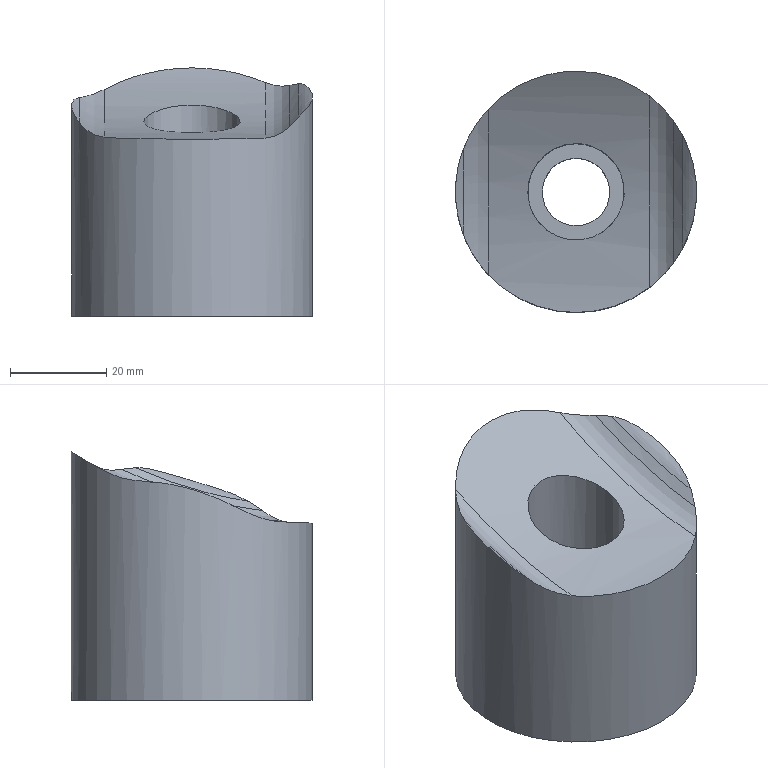Part | NX | features solid 2 | 1 solid | 11 faces | box 50 x 50 x 51.467 mm | volume 72025 mm3 | cylinder 4 | torus 3 | plane 2 | cone 2 | commonest cylinder face diameters 14 x1 20 x1 50 x1 190.6 x1
STEP:
#1=CARTESIAN_POINT('',(246.755,457.091,96.981));
#2=VERTEX_POINT('',#1);
#3=CARTESIAN_POINT('',(280.138,459.895,98.459));
#4=VERTEX_POINT('',#3);
#5=CARTESIAN_POINT('',(246.755,457.091,96.981));
#6=CARTESIAN_POINT('',(248.782,459.256,98.076));
#7=CARTESIAN_POINT('',(253.586,462.863,100.113));
#8=CARTESIAN_POINT('',(262.676,465.499,101.791));
#9=CARTESIAN_POINT('',(272.252,464.536,101.162));
#10=CARTESIAN_POINT('',(277.747,461.715,99.458));
#11=CARTESIAN_POINT('',(280.138,459.895,98.459));
#12=B_SPLINE_CURVE_WITH_KNOTS('',3,(#5,#6,#7,#8,#9,#10,#11),.UNSPECIFIED.,.F.,.F.,(4,1,1,1,4),(0.,0.009367,0.01873,0.0281,0.03747),.UNSPECIFIED.);
#13=EDGE_CURVE('',#2,#4,#12,.T.);
#14=ORIENTED_EDGE('',*,*,#13,.T.);
#15=CARTESIAN_POINT('',(285.3,454.592,97.851));
#16=VERTEX_POINT('',#15);
#17=CARTESIAN_POINT('',(280.138,459.895,98.459));
#18=CARTESIAN_POINT('',(282.045,458.445,97.663));
#19=CARTESIAN_POINT('',(283.844,456.617,97.463));
#20=CARTESIAN_POINT('',(285.3,454.592,97.851));
#21=B_SPLINE_CURVE_WITH_KNOTS('',3,(#17,#18,#19,#20),.UNSPECIFIED.,.F.,.F.,(4,4),(0.000001905,0.007488),.UNSPECIFIED.);
#22=EDGE_CURVE('',#4,#16,#21,.T.);
#23=ORIENTED_EDGE('',*,*,#22,.T.);
#24=CARTESIAN_POINT('',(287.106,451.676,98.177));
#25=VERTEX_POINT('',#24);
#26=CARTESIAN_POINT('',(285.3,454.592,97.851));
#27=CARTESIAN_POINT('',(285.965,453.667,98.029));
#28=CARTESIAN_POINT('',(286.568,452.695,98.136));
#29=CARTESIAN_POINT('',(287.106,451.676,98.177));
#30=B_SPLINE_CURVE_WITH_KNOTS('',3,(#26,#27,#28,#29),.UNSPECIFIED.,.F.,.F.,(4,4),(0.0003121,0.003757),.UNSPECIFIED.);
#31=EDGE_CURVE('',#16,#25,#30,.T.);
#32=ORIENTED_EDGE('',*,*,#31,.T.);
#33=CARTESIAN_POINT('',(287.106,428.324,91.235));
#34=VERTEX_POINT('',#33);
#35=CARTESIAN_POINT('',(287.106,428.324,91.235));
#36=CARTESIAN_POINT('',(287.985,429.988,92.248));
#37=CARTESIAN_POINT('',(289.457,433.729,93.634));
#38=CARTESIAN_POINT('',(290.244,439.786,95.413));
#39=CARTESIAN_POINT('',(289.563,445.853,97.258));
#40=CARTESIAN_POINT('',(288.105,449.785,98.252));
#41=CARTESIAN_POINT('',(287.106,451.676,98.177));
#42=B_SPLINE_CURVE_WITH_KNOTS('',3,(#35,#36,#37,#38,#39,#40,#41),.UNSPECIFIED.,.F.,.F.,(4,1,1,1,4),(0.00000349,0.006329,0.01265,0.01898,0.02531),.UNSPECIFIED.);
#43=EDGE_CURVE('',#34,#25,#42,.T.);
#44=ORIENTED_EDGE('',*,*,#43,.F.);
#45=CARTESIAN_POINT('',(285.3,425.408,89.288));
#46=VERTEX_POINT('',#45);
#47=CARTESIAN_POINT('',(287.106,428.324,91.235));
#48=CARTESIAN_POINT('',(286.564,427.298,90.611));
#49=CARTESIAN_POINT('',(285.96,426.327,89.963));
#50=CARTESIAN_POINT('',(285.3,425.408,89.288));
#51=B_SPLINE_CURVE_WITH_KNOTS('',3,(#47,#48,#49,#50),.UNSPECIFIED.,.F.,.F.,(4,4),(0.0004483,0.004392),.UNSPECIFIED.);
#52=EDGE_CURVE('',#34,#46,#51,.T.);
#53=ORIENTED_EDGE('',*,*,#52,.T.);
#54=CARTESIAN_POINT('',(280.138,420.105,86.9));
#55=VERTEX_POINT('',#54);
#56=CARTESIAN_POINT('',(285.3,425.408,89.288));
#57=CARTESIAN_POINT('',(283.974,423.564,87.935));
#58=CARTESIAN_POINT('',(282.249,421.71,87.002));
#59=CARTESIAN_POINT('',(280.138,420.105,86.9));
#60=B_SPLINE_CURVE_WITH_KNOTS('',3,(#56,#57,#58,#59),.UNSPECIFIED.,.F.,.F.,(4,4),(0.00000286,0.007823),.UNSPECIFIED.);
#61=EDGE_CURVE('',#46,#55,#60,.T.);
#62=ORIENTED_EDGE('',*,*,#61,.T.);
#63=CARTESIAN_POINT('',(246.755,422.909,87.12));
#64=VERTEX_POINT('',#63);
#65=CARTESIAN_POINT('',(280.138,420.105,86.9));
#66=CARTESIAN_POINT('',(277.683,418.236,86.781));
#67=CARTESIAN_POINT('',(272.157,415.459,86.709));
#68=CARTESIAN_POINT('',(262.859,414.519,86.711));
#69=CARTESIAN_POINT('',(253.861,416.991,86.727));
#70=CARTESIAN_POINT('',(248.861,420.661,86.91));
#71=CARTESIAN_POINT('',(246.755,422.909,87.12));
#72=B_SPLINE_CURVE_WITH_KNOTS('',3,(#65,#66,#67,#68,#69,#70,#71),.UNSPECIFIED.,.F.,.F.,(4,1,1,1,4),(0.,0.009131,0.01826,0.02739,0.03652),.UNSPECIFIED.);
#73=EDGE_CURVE('',#55,#64,#72,.T.);
#74=ORIENTED_EDGE('',*,*,#73,.T.);
#75=CARTESIAN_POINT('',(241.593,431.218,90.186));
#76=VERTEX_POINT('',#75);
#77=CARTESIAN_POINT('',(246.755,422.909,87.12));
#78=CARTESIAN_POINT('',(244.374,425.451,87.358));
#79=CARTESIAN_POINT('',(242.695,428.283,88.692));
#80=CARTESIAN_POINT('',(241.593,431.218,90.186));
#81=B_SPLINE_CURVE_WITH_KNOTS('',3,(#77,#78,#79,#80),.UNSPECIFIED.,.F.,.F.,(4,4),(0.000002101,0.01032),.UNSPECIFIED.);
#82=EDGE_CURVE('',#64,#76,#81,.T.);
#83=ORIENTED_EDGE('',*,*,#82,.T.);
#84=CARTESIAN_POINT('',(241.593,448.782,95.292));
#85=VERTEX_POINT('',#84);
#86=CARTESIAN_POINT('',(241.593,431.218,90.186));
#87=CARTESIAN_POINT('',(240.596,433.877,91.54));
#88=CARTESIAN_POINT('',(239.462,439.675,93.877));
#89=CARTESIAN_POINT('',(240.484,445.826,95.117));
#90=CARTESIAN_POINT('',(241.593,448.782,95.292));
#91=B_SPLINE_CURVE_WITH_KNOTS('',3,(#86,#87,#88,#89,#90),.UNSPECIFIED.,.F.,.F.,(4,1,4),(0.000491,0.009838,0.01918),.UNSPECIFIED.);
#92=EDGE_CURVE('',#76,#85,#91,.T.);
#93=ORIENTED_EDGE('',*,*,#92,.T.);
#94=CARTESIAN_POINT('',(241.593,448.782,95.292));
#95=CARTESIAN_POINT('',(242.774,451.928,95.478));
#96=CARTESIAN_POINT('',(244.588,454.778,95.81));
#97=CARTESIAN_POINT('',(246.755,457.091,96.981));
#98=B_SPLINE_CURVE_WITH_KNOTS('',3,(#94,#95,#96,#97),.UNSPECIFIED.,.F.,.F.,(4,4),(0.000004086,0.009949),.UNSPECIFIED.);
#99=EDGE_CURVE('',#85,#2,#98,.T.);
#100=ORIENTED_EDGE('',*,*,#99,.T.);
#101=EDGE_LOOP('',(#14,#23,#32,#44,#53,#62,#74,#83,#93,#100));
#102=FACE_BOUND('',#101,.T.);
#103=CARTESIAN_POINT('',(265.,415.,50.));
#104=VERTEX_POINT('',#103);
#105=CARTESIAN_POINT('',(265.,440.,50.));
#106=DIRECTION('',(0.,0.,1.));
#107=DIRECTION('',(0.,-1.,0.));
#108=AXIS2_PLACEMENT_3D('',#105,#106,#107);
#109=CIRCLE('',#108,25.);
#110=EDGE_CURVE('',#104,#104,#109,.T.);
#111=ORIENTED_EDGE('',*,*,#110,.T.);
#112=EDGE_LOOP('',(#111));
#113=FACE_BOUND('',#112,.T.);
#114=CARTESIAN_POINT('',(265.,440.,100.));
#115=DIRECTION('',(0.,0.,-1.));
#116=DIRECTION('',(0.,1.,0.));
#117=AXIS2_PLACEMENT_3D('',#114,#115,#116);
#118=CYLINDRICAL_SURFACE('',#117,25.);
#119=ADVANCED_FACE('',(#102,#113),#118,.T.);
#120=CARTESIAN_POINT('',(265.,433.,50.));
#121=VERTEX_POINT('',#120);
#122=CARTESIAN_POINT('',(265.,440.,50.));
#123=DIRECTION('',(0.,0.,1.));
#124=DIRECTION('',(0.,-1.,0.));
#125=AXIS2_PLACEMENT_3D('',#122,#123,#124);
#126=CIRCLE('',#125,7.);
#127=EDGE_CURVE('',#121,#121,#126,.T.);
#128=ORIENTED_EDGE('',*,*,#127,.T.);
#129=EDGE_LOOP('',(#128));
#130=FACE_BOUND('',#129,.T.);
#131=ORIENTED_EDGE('',*,*,#110,.F.);
#132=EDGE_LOOP('',(#131));
#133=FACE_BOUND('',#132,.T.);
#134=CARTESIAN_POINT('',(265.,440.,50.));
#135=DIRECTION('',(0.,0.,1.));
#136=DIRECTION('',(0.,-1.,0.));
#137=AXIS2_PLACEMENT_3D('',#134,#135,#136);
#138=PLANE('',#137);
#139=ADVANCED_FACE('',(#130,#133),#138,.F.);
#140=CARTESIAN_POINT('',(287.106,451.676,98.177));
#141=CARTESIAN_POINT('',(287.106,444.246,94.842));
#142=CARTESIAN_POINT('',(287.106,436.37,92.501));
#143=CARTESIAN_POINT('',(287.106,428.324,91.235));
#144=B_SPLINE_CURVE_WITH_KNOTS('',3,(#140,#141,#142,#143),.UNSPECIFIED.,.F.,.F.,(4,4),(0.5129,0.8199),.UNSPECIFIED.);
#145=EDGE_CURVE('',#25,#34,#144,.T.);
#146=ORIENTED_EDGE('',*,*,#145,.T.);
#147=ORIENTED_EDGE('',*,*,#43,.T.);
#148=EDGE_LOOP('',(#146,#147));
#149=FACE_BOUND('',#148,.T.);
#150=CARTESIAN_POINT('',(292.267,414.051,182.008));
#151=DIRECTION('',(-1.,0.000000001,-0.000000003));
#152=DIRECTION('',(0.000000003,0.,-1.));
#153=AXIS2_PLACEMENT_3D('',#150,#151,#152);
#154=TOROIDAL_SURFACE('',#153,98.,8.);
#155=ADVANCED_FACE('',(#149),#154,.T.);
#156=ORIENTED_EDGE('',*,*,#92,.F.);
#157=CARTESIAN_POINT('',(241.593,431.218,90.186));
#158=CARTESIAN_POINT('',(241.593,437.221,91.308));
#159=CARTESIAN_POINT('',(241.593,443.113,93.021));
#160=CARTESIAN_POINT('',(241.593,448.782,95.292));
#161=B_SPLINE_CURVE_WITH_KNOTS('',3,(#157,#158,#159,#160),.UNSPECIFIED.,.F.,.F.,(4,4),(0.2134,0.4398),.UNSPECIFIED.);
#162=EDGE_CURVE('',#76,#85,#161,.T.);
#163=ORIENTED_EDGE('',*,*,#162,.T.);
#164=EDGE_LOOP('',(#156,#163));
#165=FACE_BOUND('',#164,.T.);
#166=CARTESIAN_POINT('',(1091663.416,414.051,182.008));
#167=DIRECTION('',(1.,0.,0.));
#168=DIRECTION('',(0.,0.,1.));
#169=AXIS2_PLACEMENT_3D('',#166,#167,#168);
#170=CONICAL_SURFACE('',#169,921645.996,0.7012);
#171=ADVANCED_FACE('',(#165),#170,.F.);
#172=ORIENTED_EDGE('',*,*,#52,.F.);
#173=ORIENTED_EDGE('',*,*,#145,.F.);
#174=ORIENTED_EDGE('',*,*,#31,.F.);
#175=CARTESIAN_POINT('',(285.3,454.592,97.851));
#176=CARTESIAN_POINT('',(285.3,445.418,93.432));
#177=CARTESIAN_POINT('',(285.3,435.516,90.526));
#178=CARTESIAN_POINT('',(285.3,425.408,89.288));
#179=B_SPLINE_CURVE_WITH_KNOTS('',3,(#175,#176,#177,#178),.UNSPECIFIED.,.F.,.F.,(4,4),(0.4817,0.8593),.UNSPECIFIED.);
#180=EDGE_CURVE('',#16,#46,#179,.T.);
#181=ORIENTED_EDGE('',*,*,#180,.T.);
#182=EDGE_LOOP('',(#172,#173,#174,#181));
#183=FACE_BOUND('',#182,.T.);
#184=CARTESIAN_POINT('',(-1091136.546,414.051,182.008));
#185=DIRECTION('',(-1.,0.,0.));
#186=DIRECTION('',(0.,0.,1.));
#187=AXIS2_PLACEMENT_3D('',#184,#185,#186);
#188=CONICAL_SURFACE('',#187,921645.98,0.7012);
#189=ADVANCED_FACE('',(#183),#188,.F.);
#190=ORIENTED_EDGE('',*,*,#99,.F.);
#191=ORIENTED_EDGE('',*,*,#162,.F.);
#192=ORIENTED_EDGE('',*,*,#82,.F.);
#193=CARTESIAN_POINT('',(246.755,457.091,96.981));
#194=CARTESIAN_POINT('',(246.755,446.448,91.593));
#195=CARTESIAN_POINT('',(246.755,434.786,88.229));
#196=CARTESIAN_POINT('',(246.755,422.909,87.12));
#197=B_SPLINE_CURVE_WITH_KNOTS('',3,(#193,#194,#195,#196),.UNSPECIFIED.,.F.,.F.,(4,4),(0.459,0.8925),.UNSPECIFIED.);
#198=EDGE_CURVE('',#2,#64,#197,.T.);
#199=ORIENTED_EDGE('',*,*,#198,.F.);
#200=EDGE_LOOP('',(#190,#191,#192,#199));
#201=FACE_BOUND('',#200,.T.);
#202=CARTESIAN_POINT('',(246.755,414.051,182.008));
#203=DIRECTION('',(1.,0.000000002,-0.000000003));
#204=DIRECTION('',(0.000000003,0.,1.));
#205=AXIS2_PLACEMENT_3D('',#202,#203,#204);
#206=TOROIDAL_SURFACE('',#205,87.3,8.);
#207=ADVANCED_FACE('',(#201),#206,.F.);
#208=ORIENTED_EDGE('',*,*,#61,.F.);
#209=ORIENTED_EDGE('',*,*,#180,.F.);
#210=ORIENTED_EDGE('',*,*,#22,.F.);
#211=CARTESIAN_POINT('',(280.138,420.105,86.9));
#212=CARTESIAN_POINT('',(280.138,434.,87.785));
#213=CARTESIAN_POINT('',(280.138,447.689,91.761));
#214=CARTESIAN_POINT('',(280.138,459.895,98.459));
#215=B_SPLINE_CURVE_WITH_KNOTS('',3,(#211,#212,#213,#214),.UNSPECIFIED.,.F.,.F.,(4,4),(0.07339,0.5794),.UNSPECIFIED.);
#216=EDGE_CURVE('',#55,#4,#215,.T.);
#217=ORIENTED_EDGE('',*,*,#216,.F.);
#218=EDGE_LOOP('',(#208,#209,#210,#217));
#219=FACE_BOUND('',#218,.T.);
#220=CARTESIAN_POINT('',(280.138,414.051,182.008));
#221=DIRECTION('',(1.,0.000000001,-0.000000001));
#222=DIRECTION('',(0.000000001,0.,1.));
#223=AXIS2_PLACEMENT_3D('',#220,#221,#222);
#224=TOROIDAL_SURFACE('',#223,87.3,8.);
#225=ADVANCED_FACE('',(#219),#224,.F.);
#226=CARTESIAN_POINT('',(263.88,430.063,88.062));
#227=VERTEX_POINT('',#226);
#228=CARTESIAN_POINT('',(256.199,433.238,88.575));
#229=CARTESIAN_POINT('',(263.748,428.926,87.886));
#230=CARTESIAN_POINT('',(272.088,431.437,88.257));
#231=CARTESIAN_POINT('',(275.995,438.971,89.885));
#232=CARTESIAN_POINT('',(274.037,445.509,92.004));
#233=CARTESIAN_POINT('',(270.028,448.944,93.318));
#234=CARTESIAN_POINT('',(266.167,450.206,93.833));
#235=CARTESIAN_POINT('',(262.084,449.847,93.684));
#236=CARTESIAN_POINT('',(257.341,447.329,92.677));
#237=CARTESIAN_POINT('',(254.056,441.335,90.559));
#238=CARTESIAN_POINT('',(256.199,433.238,88.575));
#239=CARTESIAN_POINT('',(263.748,428.926,87.886));
#240=CARTESIAN_POINT('',(272.088,431.437,88.257));
#241=B_SPLINE_CURVE_WITH_KNOTS('',3,(#228,#229,#230,#231,#232,#233,#234,#235,#236,#237,#238,#239,#240),.UNSPECIFIED.,.T.,.F.,(1,1,1,1,1,1,1,1,1,1,1,1,1,1,1,1,1),(-0.02394,-0.01596,-0.007979,0.,0.007979,0.01596,0.02394,0.02792,0.03191,0.0359,0.03989,0.04787,0.05585,0.06383,0.07181,0.07979,0.08776),.UNSPECIFIED.);
#242=EDGE_CURVE('',#227,#227,#241,.T.);
#243=ORIENTED_EDGE('',*,*,#242,.F.);
#244=EDGE_LOOP('',(#243));
#245=FACE_BOUND('',#244,.T.);
#246=ORIENTED_EDGE('',*,*,#13,.F.);
#247=ORIENTED_EDGE('',*,*,#198,.T.);
#248=ORIENTED_EDGE('',*,*,#73,.F.);
#249=ORIENTED_EDGE('',*,*,#216,.T.);
#250=EDGE_LOOP('',(#246,#247,#248,#249));
#251=FACE_BOUND('',#250,.T.);
#252=CARTESIAN_POINT('',(-5999753.245,414.051,182.008));
#253=DIRECTION('',(1.,0.,0.));
#254=DIRECTION('',(0.,0.,1.));
#255=AXIS2_PLACEMENT_3D('',#252,#253,#254);
#256=CYLINDRICAL_SURFACE('',#255,95.3);
#257=ADVANCED_FACE('',(#245,#251),#256,.F.);
#258=CARTESIAN_POINT('',(265.,447.,70.));
#259=VERTEX_POINT('',#258);
#260=CARTESIAN_POINT('',(265.,440.,70.));
#261=DIRECTION('',(0.,0.,-1.));
#262=DIRECTION('',(0.,1.,0.));
#263=AXIS2_PLACEMENT_3D('',#260,#261,#262);
#264=CIRCLE('',#263,7.);
#265=EDGE_CURVE('',#259,#259,#264,.T.);
#266=ORIENTED_EDGE('',*,*,#265,.T.);
#267=EDGE_LOOP('',(#266));
#268=FACE_BOUND('',#267,.T.);
#269=CARTESIAN_POINT('',(265.,450.,70.));
#270=VERTEX_POINT('',#269);
#271=CARTESIAN_POINT('',(265.,440.,70.));
#272=DIRECTION('',(0.,0.,-1.));
#273=DIRECTION('',(0.,1.,0.));
#274=AXIS2_PLACEMENT_3D('',#271,#272,#273);
#275=CIRCLE('',#274,10.);
#276=EDGE_CURVE('',#270,#270,#275,.T.);
#277=ORIENTED_EDGE('',*,*,#276,.F.);
#278=EDGE_LOOP('',(#277));
#279=FACE_BOUND('',#278,.T.);
#280=CARTESIAN_POINT('',(265.,440.,70.));
#281=DIRECTION('',(0.,0.,-1.));
#282=DIRECTION('',(0.,1.,0.));
#283=AXIS2_PLACEMENT_3D('',#280,#281,#282);
#284=PLANE('',#283);
#285=ADVANCED_FACE('',(#268,#279),#284,.F.);
#286=ORIENTED_EDGE('',*,*,#242,.T.);
#287=EDGE_LOOP('',(#286));
#288=FACE_BOUND('',#287,.T.);
#289=ORIENTED_EDGE('',*,*,#276,.T.);
#290=EDGE_LOOP('',(#289));
#291=FACE_BOUND('',#290,.T.);
#292=CARTESIAN_POINT('',(265.,440.,150.));
#293=DIRECTION('',(0.,0.,-1.));
#294=DIRECTION('',(0.,1.,0.));
#295=AXIS2_PLACEMENT_3D('',#292,#293,#294);
#296=CYLINDRICAL_SURFACE('',#295,10.);
#297=ADVANCED_FACE('',(#288,#291),#296,.F.);
#298=ORIENTED_EDGE('',*,*,#265,.F.);
#299=EDGE_LOOP('',(#298));
#300=FACE_BOUND('',#299,.T.);
#301=ORIENTED_EDGE('',*,*,#127,.F.);
#302=EDGE_LOOP('',(#301));
#303=FACE_BOUND('',#302,.T.);
#304=CARTESIAN_POINT('',(265.,440.,70.));
#305=DIRECTION('',(0.,0.,-1.));
#306=DIRECTION('',(0.,1.,0.));
#307=AXIS2_PLACEMENT_3D('',#304,#305,#306);
#308=CYLINDRICAL_SURFACE('',#307,7.);
#309=ADVANCED_FACE('',(#300,#303),#308,.F.);
#310=CLOSED_SHELL('',(#119,#139,#155,#171,#189,#207,#225,#257,#285,#297,#309));
#311=MANIFOLD_SOLID_BREP('',#310);
#312=(LENGTH_UNIT()NAMED_UNIT(*)SI_UNIT(.MILLI.,.METRE.));
#313=UNCERTAINTY_MEASURE_WITH_UNIT(LENGTH_MEASURE(0.0508),#312,'','');
#314=(NAMED_UNIT(*)PLANE_ANGLE_UNIT()SI_UNIT($,.RADIAN.));
#315=(NAMED_UNIT(*)SI_UNIT($,.STERADIAN.)SOLID_ANGLE_UNIT());
#316=(GEOMETRIC_REPRESENTATION_CONTEXT(3)GLOBAL_UNCERTAINTY_ASSIGNED_CONTEXT((#313))GLOBAL_UNIT_ASSIGNED_CONTEXT((#312,#314,#315))REPRESENTATION_CONTEXT('',''));
#317=ADVANCED_BREP_SHAPE_REPRESENTATION('',(#311),#316);